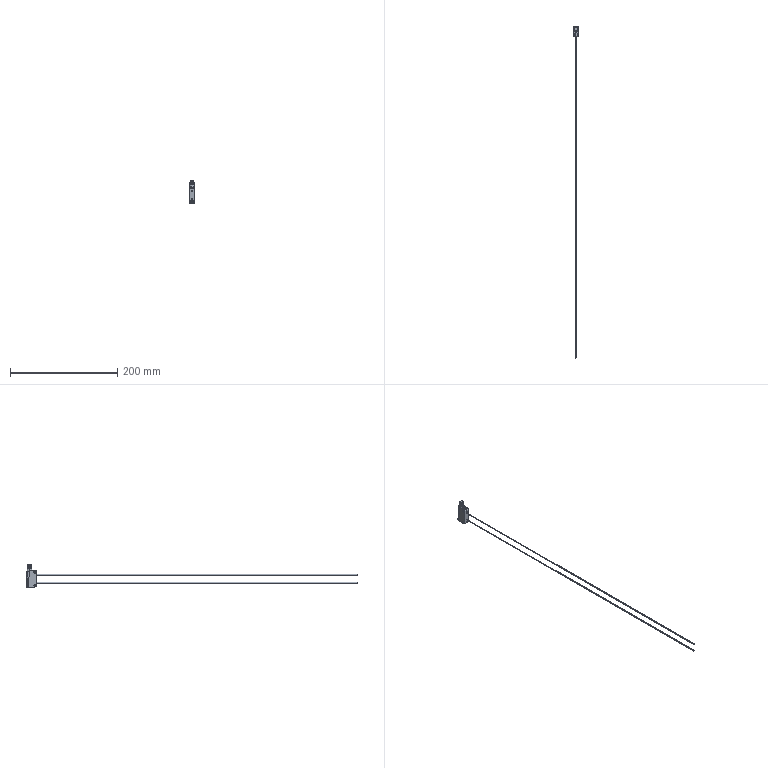Part | SolidWorks | features BaseBody 1 | 1 solid | 485 faces | box 11 x 620 x 42.399 mm | volume 8963 mm3 | plane 175 | cylinder 144 | spline 63 | torus 52 | cone 31 | sphere 20 | commonest cylinder face diameters 0.2 x68 0.6 x14 1 x12 2.4 x6 4.7 x6 4 x5